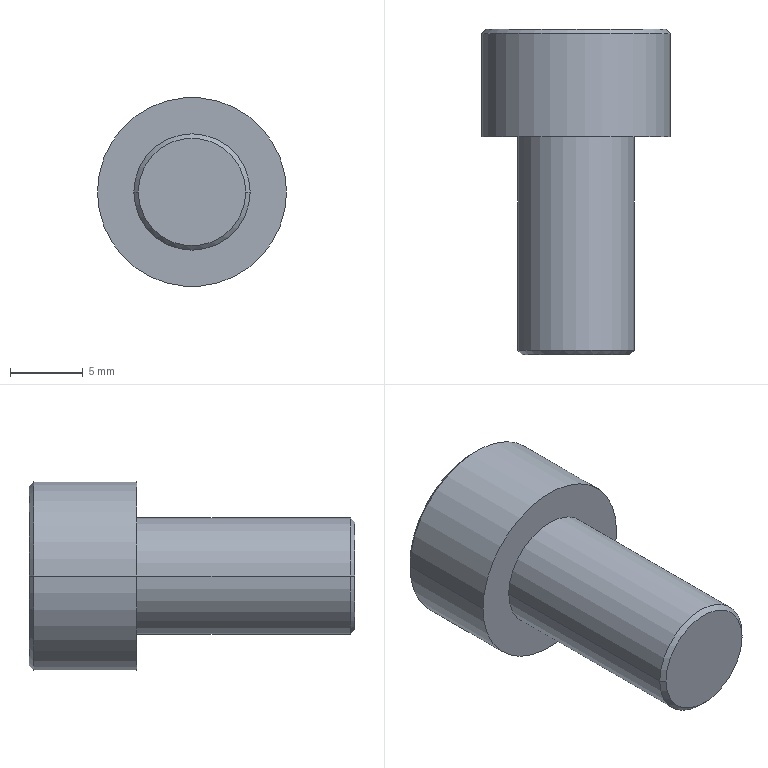Part | NX | 1 solid | 104 faces | box 13 x 22.4 x 13 mm | volume 1594 mm3 | plane 92 | cone 6 | cylinder 6 | commonest cylinder face diameters 6 x2 8 x2 13 x2